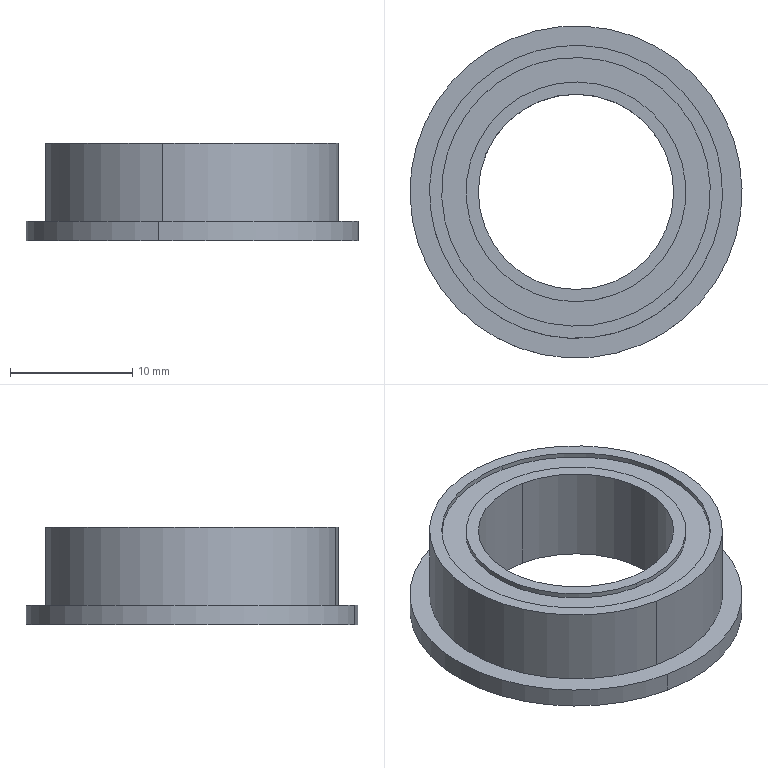Part | NX | features BREP 1 | 1 solid | 21 faces | box 27.2 x 27.2 x 8 mm | volume 2116 mm3 | cylinder 14 | plane 7 | commonest cylinder face diameters 18 x4 22 x4 16 x2 24 x2 27.2 x2
STEP:
#1=CARTESIAN_POINT('',(-58.192,157.817,11.4));
#2=VERTEX_POINT('',#1);
#3=CARTESIAN_POINT('',(-61.808,140.183,11.4));
#4=VERTEX_POINT('',#3);
#5=CARTESIAN_POINT('',(-60.,149.,11.4));
#6=DIRECTION('',(0.,0.,1.));
#7=DIRECTION('',(0.2009,0.9796,0.));
#8=AXIS2_PLACEMENT_3D('',#5,#6,#7);
#9=CIRCLE('',#8,9.);
#10=EDGE_CURVE('',#2,#4,#9,.T.);
#11=ORIENTED_EDGE('',*,*,#10,.F.);
#12=CARTESIAN_POINT('',(-58.192,157.817,11.));
#13=VERTEX_POINT('',#12);
#14=CARTESIAN_POINT('',(-58.192,157.817,11.4));
#15=DIRECTION('',(0.,0.,1.));
#16=VECTOR('',#15,1000.);
#17=LINE('',#14,#16);
#18=EDGE_CURVE('',#13,#2,#17,.T.);
#19=ORIENTED_EDGE('',*,*,#18,.F.);
#20=CARTESIAN_POINT('',(-61.808,140.183,11.));
#21=VERTEX_POINT('',#20);
#22=CARTESIAN_POINT('',(-60.,149.,11.));
#23=DIRECTION('',(0.,0.,1.));
#24=DIRECTION('',(0.2009,0.9796,0.));
#25=AXIS2_PLACEMENT_3D('',#22,#23,#24);
#26=CIRCLE('',#25,9.);
#27=EDGE_CURVE('',#13,#21,#26,.T.);
#28=ORIENTED_EDGE('',*,*,#27,.T.);
#29=CARTESIAN_POINT('',(-61.808,140.183,11.4));
#30=DIRECTION('',(0.,0.,-1.));
#31=VECTOR('',#30,1000.);
#32=LINE('',#29,#31);
#33=EDGE_CURVE('',#4,#21,#32,.T.);
#34=ORIENTED_EDGE('',*,*,#33,.F.);
#35=EDGE_LOOP('',(#11,#19,#28,#34));
#36=FACE_BOUND('',#35,.T.);
#37=CARTESIAN_POINT('',(-60.,149.,11.4));
#38=DIRECTION('',(0.,0.,-1.));
#39=DIRECTION('',(0.2009,0.9796,0.));
#40=AXIS2_PLACEMENT_3D('',#37,#38,#39);
#41=CYLINDRICAL_SURFACE('',#40,9.);
#42=ADVANCED_FACE('',(#36),#41,.T.);
#43=CARTESIAN_POINT('',(-62.21,138.224,11.4));
#44=VERTEX_POINT('',#43);
#45=CARTESIAN_POINT('',(-57.79,159.776,11.4));
#46=VERTEX_POINT('',#45);
#47=CARTESIAN_POINT('',(-60.,149.,11.4));
#48=DIRECTION('',(0.,0.,1.));
#49=DIRECTION('',(0.2009,0.9796,0.));
#50=AXIS2_PLACEMENT_3D('',#47,#48,#49);
#51=CIRCLE('',#50,11.);
#52=EDGE_CURVE('',#44,#46,#51,.T.);
#53=ORIENTED_EDGE('',*,*,#52,.T.);
#54=CARTESIAN_POINT('',(-57.79,159.776,11.));
#55=VERTEX_POINT('',#54);
#56=CARTESIAN_POINT('',(-57.79,159.776,11.4));
#57=DIRECTION('',(0.,0.,-1.));
#58=VECTOR('',#57,1000.);
#59=LINE('',#56,#58);
#60=EDGE_CURVE('',#46,#55,#59,.T.);
#61=ORIENTED_EDGE('',*,*,#60,.T.);
#62=CARTESIAN_POINT('',(-62.21,138.224,11.));
#63=VERTEX_POINT('',#62);
#64=CARTESIAN_POINT('',(-60.,149.,11.));
#65=DIRECTION('',(0.,0.,1.));
#66=DIRECTION('',(0.2009,0.9796,0.));
#67=AXIS2_PLACEMENT_3D('',#64,#65,#66);
#68=CIRCLE('',#67,11.);
#69=EDGE_CURVE('',#63,#55,#68,.T.);
#70=ORIENTED_EDGE('',*,*,#69,.F.);
#71=CARTESIAN_POINT('',(-62.21,138.224,11.4));
#72=DIRECTION('',(0.,0.,1.));
#73=VECTOR('',#72,1000.);
#74=LINE('',#71,#73);
#75=EDGE_CURVE('',#63,#44,#74,.T.);
#76=ORIENTED_EDGE('',*,*,#75,.T.);
#77=EDGE_LOOP('',(#53,#61,#70,#76));
#78=FACE_BOUND('',#77,.T.);
#79=CARTESIAN_POINT('',(-60.,149.,11.4));
#80=DIRECTION('',(0.,0.,-1.));
#81=DIRECTION('',(0.2009,0.9796,0.));
#82=AXIS2_PLACEMENT_3D('',#79,#80,#81);
#83=CYLINDRICAL_SURFACE('',#82,11.);
#84=ADVANCED_FACE('',(#78),#83,.F.);
#85=CARTESIAN_POINT('',(-58.192,157.817,18.6));
#86=VERTEX_POINT('',#85);
#87=CARTESIAN_POINT('',(-61.808,140.183,18.6));
#88=VERTEX_POINT('',#87);
#89=CARTESIAN_POINT('',(-60.,149.,18.6));
#90=DIRECTION('',(0.,0.,1.));
#91=DIRECTION('',(0.2009,0.9796,0.));
#92=AXIS2_PLACEMENT_3D('',#89,#90,#91);
#93=CIRCLE('',#92,9.);
#94=EDGE_CURVE('',#86,#88,#93,.T.);
#95=ORIENTED_EDGE('',*,*,#94,.T.);
#96=CARTESIAN_POINT('',(-61.808,140.183,19.));
#97=VERTEX_POINT('',#96);
#98=CARTESIAN_POINT('',(-61.808,140.183,18.6));
#99=DIRECTION('',(0.,0.,-1.));
#100=VECTOR('',#99,1000.);
#101=LINE('',#98,#100);
#102=EDGE_CURVE('',#97,#88,#101,.T.);
#103=ORIENTED_EDGE('',*,*,#102,.F.);
#104=CARTESIAN_POINT('',(-58.192,157.817,19.));
#105=VERTEX_POINT('',#104);
#106=CARTESIAN_POINT('',(-60.,149.,19.));
#107=DIRECTION('',(0.,0.,1.));
#108=DIRECTION('',(0.2009,0.9796,0.));
#109=AXIS2_PLACEMENT_3D('',#106,#107,#108);
#110=CIRCLE('',#109,9.);
#111=EDGE_CURVE('',#105,#97,#110,.T.);
#112=ORIENTED_EDGE('',*,*,#111,.F.);
#113=CARTESIAN_POINT('',(-58.192,157.817,18.6));
#114=DIRECTION('',(0.,0.,1.));
#115=VECTOR('',#114,1000.);
#116=LINE('',#113,#115);
#117=EDGE_CURVE('',#86,#105,#116,.T.);
#118=ORIENTED_EDGE('',*,*,#117,.F.);
#119=EDGE_LOOP('',(#95,#103,#112,#118));
#120=FACE_BOUND('',#119,.T.);
#121=CARTESIAN_POINT('',(-60.,149.,18.6));
#122=DIRECTION('',(0.,0.,1.));
#123=DIRECTION('',(-0.2009,-0.9796,0.));
#124=AXIS2_PLACEMENT_3D('',#121,#122,#123);
#125=CYLINDRICAL_SURFACE('',#124,9.);
#126=ADVANCED_FACE('',(#120),#125,.T.);
#127=CARTESIAN_POINT('',(-62.21,138.224,18.6));
#128=VERTEX_POINT('',#127);
#129=CARTESIAN_POINT('',(-57.79,159.776,18.6));
#130=VERTEX_POINT('',#129);
#131=CARTESIAN_POINT('',(-60.,149.,18.6));
#132=DIRECTION('',(0.,0.,1.));
#133=DIRECTION('',(0.2009,0.9796,0.));
#134=AXIS2_PLACEMENT_3D('',#131,#132,#133);
#135=CIRCLE('',#134,11.);
#136=EDGE_CURVE('',#128,#130,#135,.T.);
#137=ORIENTED_EDGE('',*,*,#136,.F.);
#138=CARTESIAN_POINT('',(-62.21,138.224,19.));
#139=VERTEX_POINT('',#138);
#140=CARTESIAN_POINT('',(-62.21,138.224,18.6));
#141=DIRECTION('',(0.,0.,-1.));
#142=VECTOR('',#141,1000.);
#143=LINE('',#140,#142);
#144=EDGE_CURVE('',#139,#128,#143,.T.);
#145=ORIENTED_EDGE('',*,*,#144,.F.);
#146=CARTESIAN_POINT('',(-57.79,159.776,19.));
#147=VERTEX_POINT('',#146);
#148=CARTESIAN_POINT('',(-60.,149.,19.));
#149=DIRECTION('',(0.,0.,1.));
#150=DIRECTION('',(0.2009,0.9796,0.));
#151=AXIS2_PLACEMENT_3D('',#148,#149,#150);
#152=CIRCLE('',#151,11.);
#153=EDGE_CURVE('',#139,#147,#152,.T.);
#154=ORIENTED_EDGE('',*,*,#153,.T.);
#155=CARTESIAN_POINT('',(-57.79,159.776,18.6));
#156=DIRECTION('',(0.,0.,1.));
#157=VECTOR('',#156,1000.);
#158=LINE('',#155,#157);
#159=EDGE_CURVE('',#130,#147,#158,.T.);
#160=ORIENTED_EDGE('',*,*,#159,.F.);
#161=EDGE_LOOP('',(#137,#145,#154,#160));
#162=FACE_BOUND('',#161,.T.);
#163=CARTESIAN_POINT('',(-60.,149.,18.6));
#164=DIRECTION('',(0.,0.,1.));
#165=DIRECTION('',(-0.2009,-0.9796,0.));
#166=AXIS2_PLACEMENT_3D('',#163,#164,#165);
#167=CYLINDRICAL_SURFACE('',#166,11.);
#168=ADVANCED_FACE('',(#162),#167,.F.);
#169=CARTESIAN_POINT('',(-57.268,162.323,12.6));
#170=VERTEX_POINT('',#169);
#171=CARTESIAN_POINT('',(-62.732,135.677,12.6));
#172=VERTEX_POINT('',#171);
#173=CARTESIAN_POINT('',(-60.,149.,12.6));
#174=DIRECTION('',(0.,0.,1.));
#175=DIRECTION('',(0.2009,0.9796,0.));
#176=AXIS2_PLACEMENT_3D('',#173,#174,#175);
#177=CIRCLE('',#176,13.6);
#178=EDGE_CURVE('',#170,#172,#177,.T.);
#179=ORIENTED_EDGE('',*,*,#178,.F.);
#180=CARTESIAN_POINT('',(-57.268,162.323,11.));
#181=VERTEX_POINT('',#180);
#182=CARTESIAN_POINT('',(-57.268,162.323,12.6));
#183=DIRECTION('',(0.,0.,-1.));
#184=VECTOR('',#183,1000.);
#185=LINE('',#182,#184);
#186=EDGE_CURVE('',#170,#181,#185,.T.);
#187=ORIENTED_EDGE('',*,*,#186,.T.);
#188=CARTESIAN_POINT('',(-62.732,135.677,11.));
#189=VERTEX_POINT('',#188);
#190=CARTESIAN_POINT('',(-60.,149.,11.));
#191=DIRECTION('',(0.,0.,1.));
#192=DIRECTION('',(0.2009,0.9796,0.));
#193=AXIS2_PLACEMENT_3D('',#190,#191,#192);
#194=CIRCLE('',#193,13.6);
#195=EDGE_CURVE('',#181,#189,#194,.T.);
#196=ORIENTED_EDGE('',*,*,#195,.T.);
#197=CARTESIAN_POINT('',(-62.732,135.677,12.6));
#198=DIRECTION('',(0.,0.,1.));
#199=VECTOR('',#198,1000.);
#200=LINE('',#197,#199);
#201=EDGE_CURVE('',#189,#172,#200,.T.);
#202=ORIENTED_EDGE('',*,*,#201,.T.);
#203=EDGE_LOOP('',(#179,#187,#196,#202));
#204=FACE_BOUND('',#203,.T.);
#205=CARTESIAN_POINT('',(-60.,149.,12.6));
#206=DIRECTION('',(0.,0.,-1.));
#207=DIRECTION('',(0.2009,0.9796,0.));
#208=AXIS2_PLACEMENT_3D('',#205,#206,#207);
#209=CYLINDRICAL_SURFACE('',#208,13.6);
#210=ADVANCED_FACE('',(#204),#209,.T.);
#211=CARTESIAN_POINT('',(-61.607,141.163,19.));
#212=VERTEX_POINT('',#211);
#213=CARTESIAN_POINT('',(-58.393,156.837,19.));
#214=VERTEX_POINT('',#213);
#215=CARTESIAN_POINT('',(-60.,149.,19.));
#216=DIRECTION('',(0.,0.,1.));
#217=DIRECTION('',(0.2009,0.9796,0.));
#218=AXIS2_PLACEMENT_3D('',#215,#216,#217);
#219=CIRCLE('',#218,8.);
#220=EDGE_CURVE('',#212,#214,#219,.T.);
#221=ORIENTED_EDGE('',*,*,#220,.T.);
#222=CARTESIAN_POINT('',(-58.393,156.837,11.));
#223=VERTEX_POINT('',#222);
#224=CARTESIAN_POINT('',(-58.393,156.837,19.));
#225=DIRECTION('',(0.,0.,1.));
#226=VECTOR('',#225,1000.);
#227=LINE('',#224,#226);
#228=EDGE_CURVE('',#223,#214,#227,.T.);
#229=ORIENTED_EDGE('',*,*,#228,.F.);
#230=CARTESIAN_POINT('',(-61.607,141.163,11.));
#231=VERTEX_POINT('',#230);
#232=CARTESIAN_POINT('',(-60.,149.,11.));
#233=DIRECTION('',(0.,0.,1.));
#234=DIRECTION('',(0.2009,0.9796,0.));
#235=AXIS2_PLACEMENT_3D('',#232,#233,#234);
#236=CIRCLE('',#235,8.);
#237=EDGE_CURVE('',#231,#223,#236,.T.);
#238=ORIENTED_EDGE('',*,*,#237,.F.);
#239=CARTESIAN_POINT('',(-61.607,141.163,19.));
#240=DIRECTION('',(0.,0.,-1.));
#241=VECTOR('',#240,1000.);
#242=LINE('',#239,#241);
#243=EDGE_CURVE('',#212,#231,#242,.T.);
#244=ORIENTED_EDGE('',*,*,#243,.F.);
#245=EDGE_LOOP('',(#221,#229,#238,#244));
#246=FACE_BOUND('',#245,.T.);
#247=CARTESIAN_POINT('',(-60.,149.,19.));
#248=DIRECTION('',(0.,0.,-1.));
#249=DIRECTION('',(0.2009,0.9796,0.));
#250=AXIS2_PLACEMENT_3D('',#247,#248,#249);
#251=CYLINDRICAL_SURFACE('',#250,8.);
#252=ADVANCED_FACE('',(#246),#251,.F.);
#253=CARTESIAN_POINT('',(-57.589,160.755,19.));
#254=VERTEX_POINT('',#253);
#255=CARTESIAN_POINT('',(-62.411,137.245,19.));
#256=VERTEX_POINT('',#255);
#257=CARTESIAN_POINT('',(-60.,149.,19.));
#258=DIRECTION('',(0.,0.,1.));
#259=DIRECTION('',(0.2009,0.9796,0.));
#260=AXIS2_PLACEMENT_3D('',#257,#258,#259);
#261=CIRCLE('',#260,12.);
#262=EDGE_CURVE('',#254,#256,#261,.T.);
#263=ORIENTED_EDGE('',*,*,#262,.F.);
#264=CARTESIAN_POINT('',(-57.589,160.755,12.6));
#265=VERTEX_POINT('',#264);
#266=CARTESIAN_POINT('',(-57.589,160.755,19.));
#267=DIRECTION('',(0.,0.,1.));
#268=VECTOR('',#267,1000.);
#269=LINE('',#266,#268);
#270=EDGE_CURVE('',#265,#254,#269,.T.);
#271=ORIENTED_EDGE('',*,*,#270,.F.);
#272=CARTESIAN_POINT('',(-62.411,137.245,12.6));
#273=VERTEX_POINT('',#272);
#274=CARTESIAN_POINT('',(-60.,149.,12.6));
#275=DIRECTION('',(0.,0.,1.));
#276=DIRECTION('',(0.2009,0.9796,0.));
#277=AXIS2_PLACEMENT_3D('',#274,#275,#276);
#278=CIRCLE('',#277,12.);
#279=EDGE_CURVE('',#265,#273,#278,.T.);
#280=ORIENTED_EDGE('',*,*,#279,.T.);
#281=CARTESIAN_POINT('',(-62.411,137.245,19.));
#282=DIRECTION('',(0.,0.,-1.));
#283=VECTOR('',#282,1000.);
#284=LINE('',#281,#283);
#285=EDGE_CURVE('',#256,#273,#284,.T.);
#286=ORIENTED_EDGE('',*,*,#285,.F.);
#287=EDGE_LOOP('',(#263,#271,#280,#286));
#288=FACE_BOUND('',#287,.T.);
#289=CARTESIAN_POINT('',(-60.,149.,19.));
#290=DIRECTION('',(0.,0.,-1.));
#291=DIRECTION('',(0.2009,0.9796,0.));
#292=AXIS2_PLACEMENT_3D('',#289,#290,#291);
#293=CYLINDRICAL_SURFACE('',#292,12.);
#294=ADVANCED_FACE('',(#288),#293,.T.);
#295=ORIENTED_EDGE('',*,*,#237,.T.);
#296=CARTESIAN_POINT('',(-60.,149.,11.));
#297=DIRECTION('',(0.,0.,1.));
#298=DIRECTION('',(0.2009,0.9796,0.));
#299=AXIS2_PLACEMENT_3D('',#296,#297,#298);
#300=CIRCLE('',#299,8.);
#301=EDGE_CURVE('',#223,#231,#300,.T.);
#302=ORIENTED_EDGE('',*,*,#301,.T.);
#303=EDGE_LOOP('',(#295,#302));
#304=FACE_BOUND('',#303,.T.);
#305=CARTESIAN_POINT('',(-60.,149.,11.));
#306=DIRECTION('',(0.,0.,1.));
#307=DIRECTION('',(0.2009,0.9796,0.));
#308=AXIS2_PLACEMENT_3D('',#305,#306,#307);
#309=CIRCLE('',#308,9.);
#310=EDGE_CURVE('',#21,#13,#309,.T.);
#311=ORIENTED_EDGE('',*,*,#310,.F.);
#312=ORIENTED_EDGE('',*,*,#27,.F.);
#313=EDGE_LOOP('',(#311,#312));
#314=FACE_BOUND('',#313,.T.);
#315=CARTESIAN_POINT('',(-60.,149.,11.));
#316=DIRECTION('',(0.,0.,1.));
#317=DIRECTION('',(-0.2009,-0.9796,0.));
#318=AXIS2_PLACEMENT_3D('',#315,#316,#317);
#319=PLANE('',#318);
#320=ADVANCED_FACE('',(#304,#314),#319,.F.);
#321=ORIENTED_EDGE('',*,*,#220,.F.);
#322=CARTESIAN_POINT('',(-60.,149.,19.));
#323=DIRECTION('',(0.,0.,1.));
#324=DIRECTION('',(0.2009,0.9796,0.));
#325=AXIS2_PLACEMENT_3D('',#322,#323,#324);
#326=CIRCLE('',#325,8.);
#327=EDGE_CURVE('',#214,#212,#326,.T.);
#328=ORIENTED_EDGE('',*,*,#327,.F.);
#329=EDGE_LOOP('',(#321,#328));
#330=FACE_BOUND('',#329,.T.);
#331=ORIENTED_EDGE('',*,*,#111,.T.);
#332=CARTESIAN_POINT('',(-60.,149.,19.));
#333=DIRECTION('',(0.,0.,1.));
#334=DIRECTION('',(0.2009,0.9796,0.));
#335=AXIS2_PLACEMENT_3D('',#332,#333,#334);
#336=CIRCLE('',#335,9.);
#337=EDGE_CURVE('',#97,#105,#336,.T.);
#338=ORIENTED_EDGE('',*,*,#337,.T.);
#339=EDGE_LOOP('',(#331,#338));
#340=FACE_BOUND('',#339,.T.);
#341=CARTESIAN_POINT('',(-60.,149.,19.));
#342=DIRECTION('',(0.,0.,1.));
#343=DIRECTION('',(-0.2009,-0.9796,0.));
#344=AXIS2_PLACEMENT_3D('',#341,#342,#343);
#345=PLANE('',#344);
#346=ADVANCED_FACE('',(#330,#340),#345,.T.);
#347=CARTESIAN_POINT('',(-60.,149.,19.));
#348=DIRECTION('',(0.,0.,1.));
#349=DIRECTION('',(0.2009,0.9796,0.));
#350=AXIS2_PLACEMENT_3D('',#347,#348,#349);
#351=CIRCLE('',#350,11.);
#352=EDGE_CURVE('',#147,#139,#351,.T.);
#353=ORIENTED_EDGE('',*,*,#352,.F.);
#354=ORIENTED_EDGE('',*,*,#153,.F.);
#355=EDGE_LOOP('',(#353,#354));
#356=FACE_BOUND('',#355,.T.);
#357=CARTESIAN_POINT('',(-60.,149.,19.));
#358=DIRECTION('',(0.,0.,1.));
#359=DIRECTION('',(0.2009,0.9796,0.));
#360=AXIS2_PLACEMENT_3D('',#357,#358,#359);
#361=CIRCLE('',#360,12.);
#362=EDGE_CURVE('',#256,#254,#361,.T.);
#363=ORIENTED_EDGE('',*,*,#362,.T.);
#364=ORIENTED_EDGE('',*,*,#262,.T.);
#365=EDGE_LOOP('',(#363,#364));
#366=FACE_BOUND('',#365,.T.);
#367=CARTESIAN_POINT('',(-60.,149.,19.));
#368=DIRECTION('',(0.,0.,1.));
#369=DIRECTION('',(-0.2009,-0.9796,0.));
#370=AXIS2_PLACEMENT_3D('',#367,#368,#369);
#371=PLANE('',#370);
#372=ADVANCED_FACE('',(#356,#366),#371,.T.);
#373=ORIENTED_EDGE('',*,*,#69,.T.);
#374=CARTESIAN_POINT('',(-60.,149.,11.));
#375=DIRECTION('',(0.,0.,1.));
#376=DIRECTION('',(0.2009,0.9796,0.));
#377=AXIS2_PLACEMENT_3D('',#374,#375,#376);
#378=CIRCLE('',#377,11.);
#379=EDGE_CURVE('',#55,#63,#378,.T.);
#380=ORIENTED_EDGE('',*,*,#379,.T.);
#381=EDGE_LOOP('',(#373,#380));
#382=FACE_BOUND('',#381,.T.);
#383=CARTESIAN_POINT('',(-60.,149.,11.));
#384=DIRECTION('',(0.,0.,1.));
#385=DIRECTION('',(0.2009,0.9796,0.));
#386=AXIS2_PLACEMENT_3D('',#383,#384,#385);
#387=CIRCLE('',#386,13.6);
#388=EDGE_CURVE('',#189,#181,#387,.T.);
#389=ORIENTED_EDGE('',*,*,#388,.F.);
#390=ORIENTED_EDGE('',*,*,#195,.F.);
#391=EDGE_LOOP('',(#389,#390));
#392=FACE_BOUND('',#391,.T.);
#393=CARTESIAN_POINT('',(-60.,149.,11.));
#394=DIRECTION('',(0.,0.,1.));
#395=DIRECTION('',(-0.2009,-0.9796,0.));
#396=AXIS2_PLACEMENT_3D('',#393,#394,#395);
#397=PLANE('',#396);
#398=ADVANCED_FACE('',(#382,#392),#397,.F.);
#399=ORIENTED_EDGE('',*,*,#270,.T.);
#400=ORIENTED_EDGE('',*,*,#362,.F.);
#401=ORIENTED_EDGE('',*,*,#285,.T.);
#402=CARTESIAN_POINT('',(-60.,149.,12.6));
#403=DIRECTION('',(0.,0.,1.));
#404=DIRECTION('',(0.2009,0.9796,0.));
#405=AXIS2_PLACEMENT_3D('',#402,#403,#404);
#406=CIRCLE('',#405,12.);
#407=EDGE_CURVE('',#273,#265,#406,.T.);
#408=ORIENTED_EDGE('',*,*,#407,.T.);
#409=EDGE_LOOP('',(#399,#400,#401,#408));
#410=FACE_BOUND('',#409,.T.);
#411=CARTESIAN_POINT('',(-60.,149.,19.));
#412=DIRECTION('',(0.,0.,-1.));
#413=DIRECTION('',(0.2009,0.9796,0.));
#414=AXIS2_PLACEMENT_3D('',#411,#412,#413);
#415=CYLINDRICAL_SURFACE('',#414,12.);
#416=ADVANCED_FACE('',(#410),#415,.T.);
#417=ORIENTED_EDGE('',*,*,#228,.T.);
#418=ORIENTED_EDGE('',*,*,#327,.T.);
#419=ORIENTED_EDGE('',*,*,#243,.T.);
#420=ORIENTED_EDGE('',*,*,#301,.F.);
#421=EDGE_LOOP('',(#417,#418,#419,#420));
#422=FACE_BOUND('',#421,.T.);
#423=CARTESIAN_POINT('',(-60.,149.,19.));
#424=DIRECTION('',(0.,0.,-1.));
#425=DIRECTION('',(0.2009,0.9796,0.));
#426=AXIS2_PLACEMENT_3D('',#423,#424,#425);
#427=CYLINDRICAL_SURFACE('',#426,8.);
#428=ADVANCED_FACE('',(#422),#427,.F.);
#429=CARTESIAN_POINT('',(-60.,149.,12.6));
#430=DIRECTION('',(0.,0.,1.));
#431=DIRECTION('',(0.2009,0.9796,0.));
#432=AXIS2_PLACEMENT_3D('',#429,#430,#431);
#433=CIRCLE('',#432,13.6);
#434=EDGE_CURVE('',#172,#170,#433,.T.);
#435=ORIENTED_EDGE('',*,*,#434,.T.);
#436=ORIENTED_EDGE('',*,*,#178,.T.);
#437=EDGE_LOOP('',(#435,#436));
#438=FACE_BOUND('',#437,.T.);
#439=ORIENTED_EDGE('',*,*,#407,.F.);
#440=ORIENTED_EDGE('',*,*,#279,.F.);
#441=EDGE_LOOP('',(#439,#440));
#442=FACE_BOUND('',#441,.T.);
#443=CARTESIAN_POINT('',(-60.,149.,12.6));
#444=DIRECTION('',(0.,0.,1.));
#445=DIRECTION('',(-0.2009,-0.9796,0.));
#446=AXIS2_PLACEMENT_3D('',#443,#444,#445);
#447=PLANE('',#446);
#448=ADVANCED_FACE('',(#438,#442),#447,.T.);
#449=ORIENTED_EDGE('',*,*,#186,.F.);
#450=ORIENTED_EDGE('',*,*,#434,.F.);
#451=ORIENTED_EDGE('',*,*,#201,.F.);
#452=ORIENTED_EDGE('',*,*,#388,.T.);
#453=EDGE_LOOP('',(#449,#450,#451,#452));
#454=FACE_BOUND('',#453,.T.);
#455=CARTESIAN_POINT('',(-60.,149.,12.6));
#456=DIRECTION('',(0.,0.,-1.));
#457=DIRECTION('',(0.2009,0.9796,0.));
#458=AXIS2_PLACEMENT_3D('',#455,#456,#457);
#459=CYLINDRICAL_SURFACE('',#458,13.6);
#460=ADVANCED_FACE('',(#454),#459,.T.);
#461=ORIENTED_EDGE('',*,*,#144,.T.);
#462=CARTESIAN_POINT('',(-60.,149.,18.6));
#463=DIRECTION('',(0.,0.,1.));
#464=DIRECTION('',(0.2009,0.9796,0.));
#465=AXIS2_PLACEMENT_3D('',#462,#463,#464);
#466=CIRCLE('',#465,11.);
#467=EDGE_CURVE('',#130,#128,#466,.T.);
#468=ORIENTED_EDGE('',*,*,#467,.F.);
#469=ORIENTED_EDGE('',*,*,#159,.T.);
#470=ORIENTED_EDGE('',*,*,#352,.T.);
#471=EDGE_LOOP('',(#461,#468,#469,#470));
#472=FACE_BOUND('',#471,.T.);
#473=CARTESIAN_POINT('',(-60.,149.,18.6));
#474=DIRECTION('',(0.,0.,1.));
#475=DIRECTION('',(-0.2009,-0.9796,0.));
#476=AXIS2_PLACEMENT_3D('',#473,#474,#475);
#477=CYLINDRICAL_SURFACE('',#476,11.);
#478=ADVANCED_FACE('',(#472),#477,.F.);
#479=ORIENTED_EDGE('',*,*,#94,.F.);
#480=CARTESIAN_POINT('',(-60.,149.,18.6));
#481=DIRECTION('',(0.,0.,1.));
#482=DIRECTION('',(0.2009,0.9796,0.));
#483=AXIS2_PLACEMENT_3D('',#480,#481,#482);
#484=CIRCLE('',#483,9.);
#485=EDGE_CURVE('',#88,#86,#484,.T.);
#486=ORIENTED_EDGE('',*,*,#485,.F.);
#487=EDGE_LOOP('',(#479,#486));
#488=FACE_BOUND('',#487,.T.);
#489=ORIENTED_EDGE('',*,*,#467,.T.);
#490=ORIENTED_EDGE('',*,*,#136,.T.);
#491=EDGE_LOOP('',(#489,#490));
#492=FACE_BOUND('',#491,.T.);
#493=CARTESIAN_POINT('',(-60.,149.,18.6));
#494=DIRECTION('',(0.,0.,1.));
#495=DIRECTION('',(-0.2009,-0.9796,0.));
#496=AXIS2_PLACEMENT_3D('',#493,#494,#495);
#497=PLANE('',#496);
#498=ADVANCED_FACE('',(#488,#492),#497,.T.);
#499=ORIENTED_EDGE('',*,*,#102,.T.);
#500=ORIENTED_EDGE('',*,*,#485,.T.);
#501=ORIENTED_EDGE('',*,*,#117,.T.);
#502=ORIENTED_EDGE('',*,*,#337,.F.);
#503=EDGE_LOOP('',(#499,#500,#501,#502));
#504=FACE_BOUND('',#503,.T.);
#505=CARTESIAN_POINT('',(-60.,149.,18.6));
#506=DIRECTION('',(0.,0.,1.));
#507=DIRECTION('',(-0.2009,-0.9796,0.));
#508=AXIS2_PLACEMENT_3D('',#505,#506,#507);
#509=CYLINDRICAL_SURFACE('',#508,9.);
#510=ADVANCED_FACE('',(#504),#509,.T.);
#511=ORIENTED_EDGE('',*,*,#52,.F.);
#512=CARTESIAN_POINT('',(-60.,149.,11.4));
#513=DIRECTION('',(0.,0.,1.));
#514=DIRECTION('',(0.2009,0.9796,0.));
#515=AXIS2_PLACEMENT_3D('',#512,#513,#514);
#516=CIRCLE('',#515,11.);
#517=EDGE_CURVE('',#46,#44,#516,.T.);
#518=ORIENTED_EDGE('',*,*,#517,.F.);
#519=EDGE_LOOP('',(#511,#518));
#520=FACE_BOUND('',#519,.T.);
#521=CARTESIAN_POINT('',(-60.,149.,11.4));
#522=DIRECTION('',(0.,0.,1.));
#523=DIRECTION('',(0.2009,0.9796,0.));
#524=AXIS2_PLACEMENT_3D('',#521,#522,#523);
#525=CIRCLE('',#524,9.);
#526=EDGE_CURVE('',#4,#2,#525,.T.);
#527=ORIENTED_EDGE('',*,*,#526,.T.);
#528=ORIENTED_EDGE('',*,*,#10,.T.);
#529=EDGE_LOOP('',(#527,#528));
#530=FACE_BOUND('',#529,.T.);
#531=CARTESIAN_POINT('',(-60.,149.,11.4));
#532=DIRECTION('',(0.,0.,-1.));
#533=DIRECTION('',(-0.2009,-0.9796,0.));
#534=AXIS2_PLACEMENT_3D('',#531,#532,#533);
#535=PLANE('',#534);
#536=ADVANCED_FACE('',(#520,#530),#535,.T.);
#537=ORIENTED_EDGE('',*,*,#60,.F.);
#538=ORIENTED_EDGE('',*,*,#517,.T.);
#539=ORIENTED_EDGE('',*,*,#75,.F.);
#540=ORIENTED_EDGE('',*,*,#379,.F.);
#541=EDGE_LOOP('',(#537,#538,#539,#540));
#542=FACE_BOUND('',#541,.T.);
#543=CARTESIAN_POINT('',(-60.,149.,11.4));
#544=DIRECTION('',(0.,0.,-1.));
#545=DIRECTION('',(0.2009,0.9796,0.));
#546=AXIS2_PLACEMENT_3D('',#543,#544,#545);
#547=CYLINDRICAL_SURFACE('',#546,11.);
#548=ADVANCED_FACE('',(#542),#547,.F.);
#549=ORIENTED_EDGE('',*,*,#18,.T.);
#550=ORIENTED_EDGE('',*,*,#526,.F.);
#551=ORIENTED_EDGE('',*,*,#33,.T.);
#552=ORIENTED_EDGE('',*,*,#310,.T.);
#553=EDGE_LOOP('',(#549,#550,#551,#552));
#554=FACE_BOUND('',#553,.T.);
#555=CARTESIAN_POINT('',(-60.,149.,11.4));
#556=DIRECTION('',(0.,0.,-1.));
#557=DIRECTION('',(0.2009,0.9796,0.));
#558=AXIS2_PLACEMENT_3D('',#555,#556,#557);
#559=CYLINDRICAL_SURFACE('',#558,9.);
#560=ADVANCED_FACE('',(#554),#559,.T.);
#561=CLOSED_SHELL('',(#42,#84,#126,#168,#210,#252,#294,#320,#346,#372,#398,#416,#428,#448,#460,#478,#498,#510,#536,#548,#560));
#562=MANIFOLD_SOLID_BREP('',#561);
#563=(LENGTH_UNIT()NAMED_UNIT(*)SI_UNIT(.MILLI.,.METRE.));
#564=UNCERTAINTY_MEASURE_WITH_UNIT(LENGTH_MEASURE(0.00001),#563,'','');
#565=(NAMED_UNIT(*)PLANE_ANGLE_UNIT()SI_UNIT($,.RADIAN.));
#566=(NAMED_UNIT(*)SI_UNIT($,.STERADIAN.)SOLID_ANGLE_UNIT());
#567=(GEOMETRIC_REPRESENTATION_CONTEXT(3)GLOBAL_UNCERTAINTY_ASSIGNED_CONTEXT((#564))GLOBAL_UNIT_ASSIGNED_CONTEXT((#563,#565,#566))REPRESENTATION_CONTEXT('',''));
#568=ADVANCED_BREP_SHAPE_REPRESENTATION('',(#562),#567);